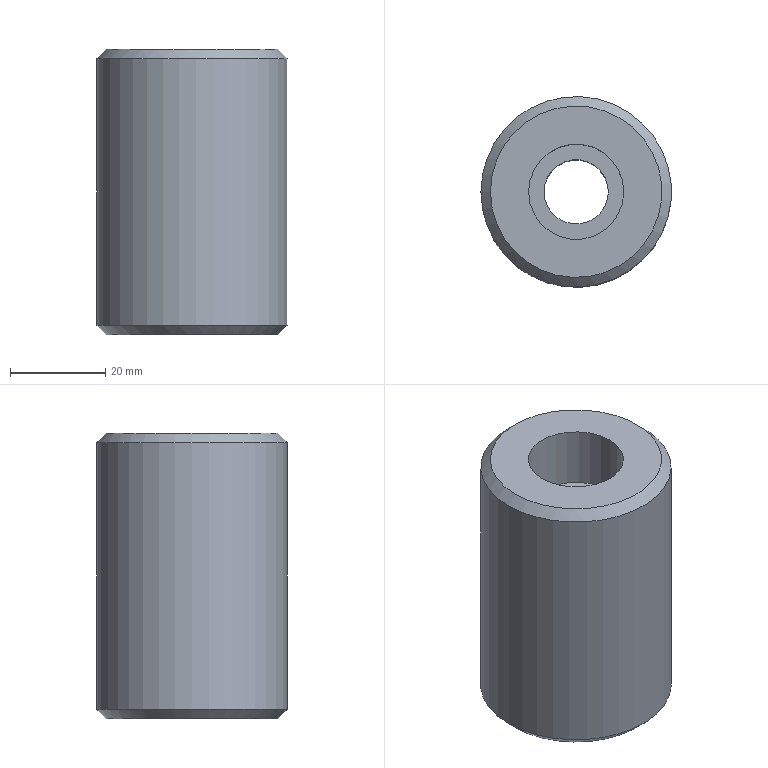Part | STEP file | solid 137 | 1 solid | 8 faces | box 40 x 40 x 60 mm | volume 64101 mm3 | plane 3 | cylinder 3 | cone 2 | commonest cylinder face diameters 13.5 x1 20 x1 40 x1